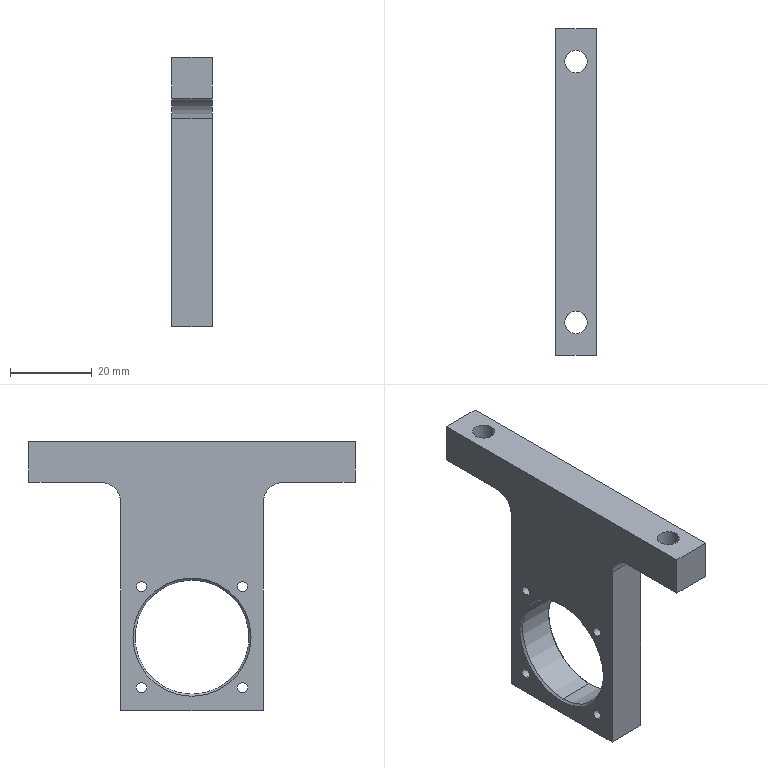Part | SolidWorks | features HoleWzd 2, Chamfer 1, Extrusion 1, Fillet 1, ICE 1 | 1 solid | 30 faces | box 10 x 80 x 66 mm | volume 20856 mm3 | cylinder 16 | plane 10 | cone 4 | commonest cylinder face diameters 2.5 x8 5.5 x4 10 x2 28 x2
STEP:
#1=CARTESIAN_POINT('',(9.5,0.,-34.));
#2=VERTEX_POINT('',#1);
#3=CARTESIAN_POINT('',(9.5,0.,-62.));
#4=VERTEX_POINT('',#3);
#5=CARTESIAN_POINT('',(9.5,0.,-48.));
#6=DIRECTION('',(1.,0.,0.));
#7=DIRECTION('',(0.,0.,1.));
#8=AXIS2_PLACEMENT_3D('',#5,#6,#7);
#9=CIRCLE('',#8,14.);
#10=EDGE_CURVE('',#2,#4,#9,.T.);
#11=ORIENTED_EDGE('',*,*,#10,.F.);
#12=CARTESIAN_POINT('',(10.,0.,-33.5));
#13=VERTEX_POINT('',#12);
#14=CARTESIAN_POINT('',(9.5,0.,-34.));
#15=DIRECTION('',(0.7071,0.,0.7071));
#16=VECTOR('',#15,1000.);
#17=LINE('',#14,#16);
#18=EDGE_CURVE('',#2,#13,#17,.T.);
#19=ORIENTED_EDGE('',*,*,#18,.T.);
#20=CARTESIAN_POINT('',(10.,0.,-62.5));
#21=VERTEX_POINT('',#20);
#22=CARTESIAN_POINT('',(10.,0.,-48.));
#23=DIRECTION('',(-1.,0.,0.));
#24=DIRECTION('',(0.,0.,1.));
#25=AXIS2_PLACEMENT_3D('',#22,#23,#24);
#26=CIRCLE('',#25,14.5);
#27=EDGE_CURVE('',#21,#13,#26,.T.);
#28=ORIENTED_EDGE('',*,*,#27,.F.);
#29=CARTESIAN_POINT('',(9.5,0.,-62.));
#30=DIRECTION('',(0.7071,0.,-0.7071));
#31=VECTOR('',#30,1000.);
#32=LINE('',#29,#31);
#33=EDGE_CURVE('',#4,#21,#32,.T.);
#34=ORIENTED_EDGE('',*,*,#33,.F.);
#35=EDGE_LOOP('',(#11,#19,#28,#34));
#36=FACE_OUTER_BOUND('',#35,.T.);
#37=CARTESIAN_POINT('',(9.5,0.,-48.));
#38=DIRECTION('',(1.,0.,0.));
#39=DIRECTION('',(0.,0.,-1.));
#40=AXIS2_PLACEMENT_3D('',#37,#38,#39);
#41=CONICAL_SURFACE('',#40,14.,0.7854);
#42=ADVANCED_FACE('',(#36),#41,.F.);
#43=CARTESIAN_POINT('',(0.5,0.,-62.));
#44=VERTEX_POINT('',#43);
#45=CARTESIAN_POINT('',(0.5,0.,-34.));
#46=VERTEX_POINT('',#45);
#47=CARTESIAN_POINT('',(0.5,0.,-48.));
#48=DIRECTION('',(-1.,0.,0.));
#49=DIRECTION('',(0.,0.,1.));
#50=AXIS2_PLACEMENT_3D('',#47,#48,#49);
#51=CIRCLE('',#50,14.);
#52=EDGE_CURVE('',#44,#46,#51,.T.);
#53=ORIENTED_EDGE('',*,*,#52,.F.);
#54=CARTESIAN_POINT('',(0.,0.,-62.5));
#55=VERTEX_POINT('',#54);
#56=CARTESIAN_POINT('',(0.,0.,-62.5));
#57=DIRECTION('',(-0.7071,0.,-0.7071));
#58=VECTOR('',#57,1000.);
#59=LINE('',#56,#58);
#60=EDGE_CURVE('',#44,#55,#59,.T.);
#61=ORIENTED_EDGE('',*,*,#60,.T.);
#62=CARTESIAN_POINT('',(0.,0.,-33.5));
#63=VERTEX_POINT('',#62);
#64=CARTESIAN_POINT('',(0.,0.,-48.));
#65=DIRECTION('',(1.,0.,0.));
#66=DIRECTION('',(0.,0.,1.));
#67=AXIS2_PLACEMENT_3D('',#64,#65,#66);
#68=CIRCLE('',#67,14.5);
#69=EDGE_CURVE('',#63,#55,#68,.T.);
#70=ORIENTED_EDGE('',*,*,#69,.F.);
#71=CARTESIAN_POINT('',(0.,0.,-33.5));
#72=DIRECTION('',(-0.7071,0.,0.7071));
#73=VECTOR('',#72,1000.);
#74=LINE('',#71,#73);
#75=EDGE_CURVE('',#46,#63,#74,.T.);
#76=ORIENTED_EDGE('',*,*,#75,.F.);
#77=EDGE_LOOP('',(#53,#61,#70,#76));
#78=FACE_OUTER_BOUND('',#77,.T.);
#79=CARTESIAN_POINT('',(0.,0.,-48.));
#80=DIRECTION('',(-1.,0.,0.));
#81=DIRECTION('',(0.,0.,1.));
#82=AXIS2_PLACEMENT_3D('',#79,#80,#81);
#83=CONICAL_SURFACE('',#82,14.5,0.7854);
#84=ADVANCED_FACE('',(#78),#83,.F.);
#85=CARTESIAN_POINT('',(0.,12.374,-34.376));
#86=VERTEX_POINT('',#85);
#87=CARTESIAN_POINT('',(0.,12.374,-36.876));
#88=VERTEX_POINT('',#87);
#89=CARTESIAN_POINT('',(0.,12.374,-35.626));
#90=DIRECTION('',(1.,0.,0.));
#91=DIRECTION('',(0.,0.,-1.));
#92=AXIS2_PLACEMENT_3D('',#89,#90,#91);
#93=CIRCLE('',#92,1.25);
#94=EDGE_CURVE('',#86,#88,#93,.T.);
#95=ORIENTED_EDGE('',*,*,#94,.F.);
#96=CARTESIAN_POINT('',(10.,12.374,-34.376));
#97=VERTEX_POINT('',#96);
#98=CARTESIAN_POINT('',(10.,12.374,-34.376));
#99=DIRECTION('',(1.,0.,0.));
#100=VECTOR('',#99,1000.);
#101=LINE('',#98,#100);
#102=EDGE_CURVE('',#86,#97,#101,.T.);
#103=ORIENTED_EDGE('',*,*,#102,.T.);
#104=CARTESIAN_POINT('',(10.,12.374,-36.876));
#105=VERTEX_POINT('',#104);
#106=CARTESIAN_POINT('',(10.,12.374,-35.626));
#107=DIRECTION('',(1.,0.,0.));
#108=DIRECTION('',(0.,0.,-1.));
#109=AXIS2_PLACEMENT_3D('',#106,#107,#108);
#110=CIRCLE('',#109,1.25);
#111=EDGE_CURVE('',#97,#105,#110,.T.);
#112=ORIENTED_EDGE('',*,*,#111,.T.);
#113=CARTESIAN_POINT('',(10.,12.374,-36.876));
#114=DIRECTION('',(1.,0.,0.));
#115=VECTOR('',#114,1000.);
#116=LINE('',#113,#115);
#117=EDGE_CURVE('',#88,#105,#116,.T.);
#118=ORIENTED_EDGE('',*,*,#117,.F.);
#119=EDGE_LOOP('',(#95,#103,#112,#118));
#120=FACE_OUTER_BOUND('',#119,.T.);
#121=CARTESIAN_POINT('',(10.,12.374,-35.626));
#122=DIRECTION('',(1.,0.,0.));
#123=DIRECTION('',(0.,0.,-1.));
#124=AXIS2_PLACEMENT_3D('',#121,#122,#123);
#125=CYLINDRICAL_SURFACE('',#124,1.25);
#126=ADVANCED_FACE('',(#120),#125,.F.);
#127=CARTESIAN_POINT('',(0.,12.374,-59.124));
#128=VERTEX_POINT('',#127);
#129=CARTESIAN_POINT('',(0.,12.374,-61.624));
#130=VERTEX_POINT('',#129);
#131=CARTESIAN_POINT('',(0.,12.374,-60.374));
#132=DIRECTION('',(1.,0.,0.));
#133=DIRECTION('',(0.,0.,-1.));
#134=AXIS2_PLACEMENT_3D('',#131,#132,#133);
#135=CIRCLE('',#134,1.25);
#136=EDGE_CURVE('',#128,#130,#135,.T.);
#137=ORIENTED_EDGE('',*,*,#136,.F.);
#138=CARTESIAN_POINT('',(10.,12.374,-59.124));
#139=VERTEX_POINT('',#138);
#140=CARTESIAN_POINT('',(10.,12.374,-59.124));
#141=DIRECTION('',(1.,0.,0.));
#142=VECTOR('',#141,1000.);
#143=LINE('',#140,#142);
#144=EDGE_CURVE('',#128,#139,#143,.T.);
#145=ORIENTED_EDGE('',*,*,#144,.T.);
#146=CARTESIAN_POINT('',(10.,12.374,-61.624));
#147=VERTEX_POINT('',#146);
#148=CARTESIAN_POINT('',(10.,12.374,-60.374));
#149=DIRECTION('',(1.,0.,0.));
#150=DIRECTION('',(0.,0.,-1.));
#151=AXIS2_PLACEMENT_3D('',#148,#149,#150);
#152=CIRCLE('',#151,1.25);
#153=EDGE_CURVE('',#139,#147,#152,.T.);
#154=ORIENTED_EDGE('',*,*,#153,.T.);
#155=CARTESIAN_POINT('',(10.,12.374,-61.624));
#156=DIRECTION('',(1.,0.,0.));
#157=VECTOR('',#156,1000.);
#158=LINE('',#155,#157);
#159=EDGE_CURVE('',#130,#147,#158,.T.);
#160=ORIENTED_EDGE('',*,*,#159,.F.);
#161=EDGE_LOOP('',(#137,#145,#154,#160));
#162=FACE_OUTER_BOUND('',#161,.T.);
#163=CARTESIAN_POINT('',(10.,12.374,-60.374));
#164=DIRECTION('',(1.,0.,0.));
#165=DIRECTION('',(0.,0.,-1.));
#166=AXIS2_PLACEMENT_3D('',#163,#164,#165);
#167=CYLINDRICAL_SURFACE('',#166,1.25);
#168=ADVANCED_FACE('',(#162),#167,.F.);
#169=CARTESIAN_POINT('',(0.,-12.374,-59.124));
#170=VERTEX_POINT('',#169);
#171=CARTESIAN_POINT('',(0.,-12.374,-61.624));
#172=VERTEX_POINT('',#171);
#173=CARTESIAN_POINT('',(0.,-12.374,-60.374));
#174=DIRECTION('',(1.,0.,0.));
#175=DIRECTION('',(0.,0.,-1.));
#176=AXIS2_PLACEMENT_3D('',#173,#174,#175);
#177=CIRCLE('',#176,1.25);
#178=EDGE_CURVE('',#170,#172,#177,.T.);
#179=ORIENTED_EDGE('',*,*,#178,.F.);
#180=CARTESIAN_POINT('',(10.,-12.374,-59.124));
#181=VERTEX_POINT('',#180);
#182=CARTESIAN_POINT('',(10.,-12.374,-59.124));
#183=DIRECTION('',(1.,0.,0.));
#184=VECTOR('',#183,1000.);
#185=LINE('',#182,#184);
#186=EDGE_CURVE('',#170,#181,#185,.T.);
#187=ORIENTED_EDGE('',*,*,#186,.T.);
#188=CARTESIAN_POINT('',(10.,-12.374,-61.624));
#189=VERTEX_POINT('',#188);
#190=CARTESIAN_POINT('',(10.,-12.374,-60.374));
#191=DIRECTION('',(1.,0.,0.));
#192=DIRECTION('',(0.,0.,-1.));
#193=AXIS2_PLACEMENT_3D('',#190,#191,#192);
#194=CIRCLE('',#193,1.25);
#195=EDGE_CURVE('',#181,#189,#194,.T.);
#196=ORIENTED_EDGE('',*,*,#195,.T.);
#197=CARTESIAN_POINT('',(10.,-12.374,-61.624));
#198=DIRECTION('',(1.,0.,0.));
#199=VECTOR('',#198,1000.);
#200=LINE('',#197,#199);
#201=EDGE_CURVE('',#172,#189,#200,.T.);
#202=ORIENTED_EDGE('',*,*,#201,.F.);
#203=EDGE_LOOP('',(#179,#187,#196,#202));
#204=FACE_OUTER_BOUND('',#203,.T.);
#205=CARTESIAN_POINT('',(10.,-12.374,-60.374));
#206=DIRECTION('',(1.,0.,0.));
#207=DIRECTION('',(0.,0.,-1.));
#208=AXIS2_PLACEMENT_3D('',#205,#206,#207);
#209=CYLINDRICAL_SURFACE('',#208,1.25);
#210=ADVANCED_FACE('',(#204),#209,.F.);
#211=CARTESIAN_POINT('',(0.,-12.374,-34.376));
#212=VERTEX_POINT('',#211);
#213=CARTESIAN_POINT('',(0.,-12.374,-36.876));
#214=VERTEX_POINT('',#213);
#215=CARTESIAN_POINT('',(0.,-12.374,-35.626));
#216=DIRECTION('',(1.,0.,0.));
#217=DIRECTION('',(0.,0.,-1.));
#218=AXIS2_PLACEMENT_3D('',#215,#216,#217);
#219=CIRCLE('',#218,1.25);
#220=EDGE_CURVE('',#212,#214,#219,.T.);
#221=ORIENTED_EDGE('',*,*,#220,.F.);
#222=CARTESIAN_POINT('',(10.,-12.374,-34.376));
#223=VERTEX_POINT('',#222);
#224=CARTESIAN_POINT('',(10.,-12.374,-34.376));
#225=DIRECTION('',(1.,0.,0.));
#226=VECTOR('',#225,1000.);
#227=LINE('',#224,#226);
#228=EDGE_CURVE('',#212,#223,#227,.T.);
#229=ORIENTED_EDGE('',*,*,#228,.T.);
#230=CARTESIAN_POINT('',(10.,-12.374,-36.876));
#231=VERTEX_POINT('',#230);
#232=CARTESIAN_POINT('',(10.,-12.374,-35.626));
#233=DIRECTION('',(1.,0.,0.));
#234=DIRECTION('',(0.,0.,-1.));
#235=AXIS2_PLACEMENT_3D('',#232,#233,#234);
#236=CIRCLE('',#235,1.25);
#237=EDGE_CURVE('',#223,#231,#236,.T.);
#238=ORIENTED_EDGE('',*,*,#237,.T.);
#239=CARTESIAN_POINT('',(10.,-12.374,-36.876));
#240=DIRECTION('',(1.,0.,0.));
#241=VECTOR('',#240,1000.);
#242=LINE('',#239,#241);
#243=EDGE_CURVE('',#214,#231,#242,.T.);
#244=ORIENTED_EDGE('',*,*,#243,.F.);
#245=EDGE_LOOP('',(#221,#229,#238,#244));
#246=FACE_OUTER_BOUND('',#245,.T.);
#247=CARTESIAN_POINT('',(10.,-12.374,-35.626));
#248=DIRECTION('',(1.,0.,0.));
#249=DIRECTION('',(0.,0.,-1.));
#250=AXIS2_PLACEMENT_3D('',#247,#248,#249);
#251=CYLINDRICAL_SURFACE('',#250,1.25);
#252=ADVANCED_FACE('',(#246),#251,.F.);
#253=CARTESIAN_POINT('',(2.25,32.,-10.));
#254=VERTEX_POINT('',#253);
#255=CARTESIAN_POINT('',(7.75,32.,-10.));
#256=VERTEX_POINT('',#255);
#257=CARTESIAN_POINT('',(5.,32.,-10.));
#258=DIRECTION('',(0.,0.,1.));
#259=DIRECTION('',(1.,0.,0.));
#260=AXIS2_PLACEMENT_3D('',#257,#258,#259);
#261=CIRCLE('',#260,2.75);
#262=EDGE_CURVE('',#254,#256,#261,.T.);
#263=ORIENTED_EDGE('',*,*,#262,.F.);
#264=CARTESIAN_POINT('',(2.25,32.,0.));
#265=VERTEX_POINT('',#264);
#266=CARTESIAN_POINT('',(2.25,32.,0.));
#267=DIRECTION('',(0.,0.,1.));
#268=VECTOR('',#267,1000.);
#269=LINE('',#266,#268);
#270=EDGE_CURVE('',#254,#265,#269,.T.);
#271=ORIENTED_EDGE('',*,*,#270,.T.);
#272=CARTESIAN_POINT('',(7.75,32.,0.));
#273=VERTEX_POINT('',#272);
#274=CARTESIAN_POINT('',(5.,32.,0.));
#275=DIRECTION('',(0.,0.,1.));
#276=DIRECTION('',(1.,0.,0.));
#277=AXIS2_PLACEMENT_3D('',#274,#275,#276);
#278=CIRCLE('',#277,2.75);
#279=EDGE_CURVE('',#265,#273,#278,.T.);
#280=ORIENTED_EDGE('',*,*,#279,.T.);
#281=CARTESIAN_POINT('',(7.75,32.,0.));
#282=DIRECTION('',(0.,0.,1.));
#283=VECTOR('',#282,1000.);
#284=LINE('',#281,#283);
#285=EDGE_CURVE('',#256,#273,#284,.T.);
#286=ORIENTED_EDGE('',*,*,#285,.F.);
#287=EDGE_LOOP('',(#263,#271,#280,#286));
#288=FACE_OUTER_BOUND('',#287,.T.);
#289=CARTESIAN_POINT('',(5.,32.,0.));
#290=DIRECTION('',(0.,0.,1.));
#291=DIRECTION('',(1.,0.,0.));
#292=AXIS2_PLACEMENT_3D('',#289,#290,#291);
#293=CYLINDRICAL_SURFACE('',#292,2.75);
#294=ADVANCED_FACE('',(#288),#293,.F.);
#295=CARTESIAN_POINT('',(2.25,-32.,-10.));
#296=VERTEX_POINT('',#295);
#297=CARTESIAN_POINT('',(7.75,-32.,-10.));
#298=VERTEX_POINT('',#297);
#299=CARTESIAN_POINT('',(5.,-32.,-10.));
#300=DIRECTION('',(0.,0.,1.));
#301=DIRECTION('',(1.,0.,0.));
#302=AXIS2_PLACEMENT_3D('',#299,#300,#301);
#303=CIRCLE('',#302,2.75);
#304=EDGE_CURVE('',#296,#298,#303,.T.);
#305=ORIENTED_EDGE('',*,*,#304,.F.);
#306=CARTESIAN_POINT('',(2.25,-32.,0.));
#307=VERTEX_POINT('',#306);
#308=CARTESIAN_POINT('',(2.25,-32.,0.));
#309=DIRECTION('',(0.,0.,1.));
#310=VECTOR('',#309,1000.);
#311=LINE('',#308,#310);
#312=EDGE_CURVE('',#296,#307,#311,.T.);
#313=ORIENTED_EDGE('',*,*,#312,.T.);
#314=CARTESIAN_POINT('',(7.75,-32.,0.));
#315=VERTEX_POINT('',#314);
#316=CARTESIAN_POINT('',(5.,-32.,0.));
#317=DIRECTION('',(0.,0.,1.));
#318=DIRECTION('',(1.,0.,0.));
#319=AXIS2_PLACEMENT_3D('',#316,#317,#318);
#320=CIRCLE('',#319,2.75);
#321=EDGE_CURVE('',#307,#315,#320,.T.);
#322=ORIENTED_EDGE('',*,*,#321,.T.);
#323=CARTESIAN_POINT('',(7.75,-32.,0.));
#324=DIRECTION('',(0.,0.,1.));
#325=VECTOR('',#324,1000.);
#326=LINE('',#323,#325);
#327=EDGE_CURVE('',#298,#315,#326,.T.);
#328=ORIENTED_EDGE('',*,*,#327,.F.);
#329=EDGE_LOOP('',(#305,#313,#322,#328));
#330=FACE_OUTER_BOUND('',#329,.T.);
#331=CARTESIAN_POINT('',(5.,-32.,0.));
#332=DIRECTION('',(0.,0.,1.));
#333=DIRECTION('',(1.,0.,0.));
#334=AXIS2_PLACEMENT_3D('',#331,#332,#333);
#335=CYLINDRICAL_SURFACE('',#334,2.75);
#336=ADVANCED_FACE('',(#330),#335,.F.);
#337=ORIENTED_EDGE('',*,*,#52,.T.);
#338=CARTESIAN_POINT('',(0.,0.,-34.));
#339=DIRECTION('',(1.,0.,0.));
#340=VECTOR('',#339,1000.);
#341=LINE('',#338,#340);
#342=EDGE_CURVE('',#46,#2,#341,.T.);
#343=ORIENTED_EDGE('',*,*,#342,.T.);
#344=ORIENTED_EDGE('',*,*,#10,.T.);
#345=CARTESIAN_POINT('',(0.,0.,-62.));
#346=DIRECTION('',(1.,0.,0.));
#347=VECTOR('',#346,1000.);
#348=LINE('',#345,#347);
#349=EDGE_CURVE('',#44,#4,#348,.T.);
#350=ORIENTED_EDGE('',*,*,#349,.F.);
#351=EDGE_LOOP('',(#337,#343,#344,#350));
#352=FACE_OUTER_BOUND('',#351,.T.);
#353=CARTESIAN_POINT('',(0.,0.,-48.));
#354=DIRECTION('',(1.,0.,0.));
#355=DIRECTION('',(0.,0.,-1.));
#356=AXIS2_PLACEMENT_3D('',#353,#354,#355);
#357=CYLINDRICAL_SURFACE('',#356,14.);
#358=ADVANCED_FACE('',(#352),#357,.F.);
#359=CARTESIAN_POINT('',(0.,-40.,0.));
#360=VERTEX_POINT('',#359);
#361=CARTESIAN_POINT('',(0.,-40.,-10.));
#362=VERTEX_POINT('',#361);
#363=CARTESIAN_POINT('',(0.,-40.,-10.));
#364=DIRECTION('',(0.,0.,-1.));
#365=VECTOR('',#364,1000.);
#366=LINE('',#363,#365);
#367=EDGE_CURVE('',#360,#362,#366,.T.);
#368=ORIENTED_EDGE('',*,*,#367,.T.);
#369=CARTESIAN_POINT('',(10.,-40.,-10.));
#370=VERTEX_POINT('',#369);
#371=CARTESIAN_POINT('',(10.,-40.,-10.));
#372=DIRECTION('',(-1.,0.,0.));
#373=VECTOR('',#372,1000.);
#374=LINE('',#371,#373);
#375=EDGE_CURVE('',#370,#362,#374,.T.);
#376=ORIENTED_EDGE('',*,*,#375,.F.);
#377=CARTESIAN_POINT('',(10.,-40.,0.));
#378=VERTEX_POINT('',#377);
#379=CARTESIAN_POINT('',(10.,-40.,-10.));
#380=DIRECTION('',(0.,0.,-1.));
#381=VECTOR('',#380,1000.);
#382=LINE('',#379,#381);
#383=EDGE_CURVE('',#378,#370,#382,.T.);
#384=ORIENTED_EDGE('',*,*,#383,.F.);
#385=CARTESIAN_POINT('',(10.,-40.,0.));
#386=DIRECTION('',(-1.,0.,0.));
#387=VECTOR('',#386,1000.);
#388=LINE('',#385,#387);
#389=EDGE_CURVE('',#378,#360,#388,.T.);
#390=ORIENTED_EDGE('',*,*,#389,.T.);
#391=EDGE_LOOP('',(#368,#376,#384,#390));
#392=FACE_OUTER_BOUND('',#391,.T.);
#393=CARTESIAN_POINT('',(10.,-40.,-10.));
#394=DIRECTION('',(0.,1.,0.));
#395=DIRECTION('',(0.,0.,1.));
#396=AXIS2_PLACEMENT_3D('',#393,#394,#395);
#397=PLANE('',#396);
#398=ADVANCED_FACE('',(#392),#397,.F.);
#399=CARTESIAN_POINT('',(5.,-32.,-10.));
#400=DIRECTION('',(0.,0.,1.));
#401=DIRECTION('',(1.,0.,0.));
#402=AXIS2_PLACEMENT_3D('',#399,#400,#401);
#403=CIRCLE('',#402,2.75);
#404=EDGE_CURVE('',#298,#296,#403,.T.);
#405=ORIENTED_EDGE('',*,*,#404,.T.);
#406=ORIENTED_EDGE('',*,*,#304,.T.);
#407=EDGE_LOOP('',(#405,#406));
#408=FACE_BOUND('',#407,.T.);
#409=CARTESIAN_POINT('',(0.,-22.5,-10.));
#410=VERTEX_POINT('',#409);
#411=CARTESIAN_POINT('',(0.,-17.5,-10.));
#412=DIRECTION('',(0.,1.,0.));
#413=VECTOR('',#412,1000.);
#414=LINE('',#411,#413);
#415=EDGE_CURVE('',#362,#410,#414,.T.);
#416=ORIENTED_EDGE('',*,*,#415,.T.);
#417=CARTESIAN_POINT('',(10.,-22.5,-10.));
#418=VERTEX_POINT('',#417);
#419=CARTESIAN_POINT('',(10.,-22.5,-10.));
#420=DIRECTION('',(1.,0.,0.));
#421=VECTOR('',#420,1000.);
#422=LINE('',#419,#421);
#423=EDGE_CURVE('',#410,#418,#422,.T.);
#424=ORIENTED_EDGE('',*,*,#423,.T.);
#425=CARTESIAN_POINT('',(10.,-17.5,-10.));
#426=DIRECTION('',(0.,1.,0.));
#427=VECTOR('',#426,1000.);
#428=LINE('',#425,#427);
#429=EDGE_CURVE('',#370,#418,#428,.T.);
#430=ORIENTED_EDGE('',*,*,#429,.F.);
#431=ORIENTED_EDGE('',*,*,#375,.T.);
#432=EDGE_LOOP('',(#416,#424,#430,#431));
#433=FACE_OUTER_BOUND('',#432,.T.);
#434=CARTESIAN_POINT('',(10.,-17.5,-10.));
#435=DIRECTION('',(0.,0.,1.));
#436=DIRECTION('',(1.,0.,0.));
#437=AXIS2_PLACEMENT_3D('',#434,#435,#436);
#438=PLANE('',#437);
#439=ADVANCED_FACE('',(#408,#433),#438,.F.);
#440=CARTESIAN_POINT('',(10.,-17.5,-15.));
#441=VERTEX_POINT('',#440);
#442=CARTESIAN_POINT('',(10.,-17.5,-66.));
#443=VERTEX_POINT('',#442);
#444=CARTESIAN_POINT('',(10.,-17.5,-66.));
#445=DIRECTION('',(0.,0.,-1.));
#446=VECTOR('',#445,1000.);
#447=LINE('',#444,#446);
#448=EDGE_CURVE('',#441,#443,#447,.T.);
#449=ORIENTED_EDGE('',*,*,#448,.F.);
#450=CARTESIAN_POINT('',(0.,-17.5,-15.));
#451=VERTEX_POINT('',#450);
#452=CARTESIAN_POINT('',(0.,-17.5,-15.));
#453=DIRECTION('',(-1.,0.,0.));
#454=VECTOR('',#453,1000.);
#455=LINE('',#452,#454);
#456=EDGE_CURVE('',#441,#451,#455,.T.);
#457=ORIENTED_EDGE('',*,*,#456,.T.);
#458=CARTESIAN_POINT('',(0.,-17.5,-66.));
#459=VERTEX_POINT('',#458);
#460=CARTESIAN_POINT('',(0.,-17.5,-66.));
#461=DIRECTION('',(0.,0.,-1.));
#462=VECTOR('',#461,1000.);
#463=LINE('',#460,#462);
#464=EDGE_CURVE('',#451,#459,#463,.T.);
#465=ORIENTED_EDGE('',*,*,#464,.T.);
#466=CARTESIAN_POINT('',(10.,-17.5,-66.));
#467=DIRECTION('',(-1.,0.,0.));
#468=VECTOR('',#467,1000.);
#469=LINE('',#466,#468);
#470=EDGE_CURVE('',#443,#459,#469,.T.);
#471=ORIENTED_EDGE('',*,*,#470,.F.);
#472=EDGE_LOOP('',(#449,#457,#465,#471));
#473=FACE_OUTER_BOUND('',#472,.T.);
#474=CARTESIAN_POINT('',(10.,-17.5,-66.));
#475=DIRECTION('',(0.,1.,0.));
#476=DIRECTION('',(0.,0.,1.));
#477=AXIS2_PLACEMENT_3D('',#474,#475,#476);
#478=PLANE('',#477);
#479=ADVANCED_FACE('',(#473),#478,.F.);
#480=CARTESIAN_POINT('',(0.,17.5,-66.));
#481=VERTEX_POINT('',#480);
#482=CARTESIAN_POINT('',(0.,17.5,-66.));
#483=DIRECTION('',(0.,1.,0.));
#484=VECTOR('',#483,1000.);
#485=LINE('',#482,#484);
#486=EDGE_CURVE('',#459,#481,#485,.T.);
#487=ORIENTED_EDGE('',*,*,#486,.T.);
#488=CARTESIAN_POINT('',(10.,17.5,-66.));
#489=VERTEX_POINT('',#488);
#490=CARTESIAN_POINT('',(10.,17.5,-66.));
#491=DIRECTION('',(-1.,0.,0.));
#492=VECTOR('',#491,1000.);
#493=LINE('',#490,#492);
#494=EDGE_CURVE('',#489,#481,#493,.T.);
#495=ORIENTED_EDGE('',*,*,#494,.F.);
#496=CARTESIAN_POINT('',(10.,17.5,-66.));
#497=DIRECTION('',(0.,1.,0.));
#498=VECTOR('',#497,1000.);
#499=LINE('',#496,#498);
#500=EDGE_CURVE('',#443,#489,#499,.T.);
#501=ORIENTED_EDGE('',*,*,#500,.F.);
#502=ORIENTED_EDGE('',*,*,#470,.T.);
#503=EDGE_LOOP('',(#487,#495,#501,#502));
#504=FACE_OUTER_BOUND('',#503,.T.);
#505=CARTESIAN_POINT('',(10.,17.5,-66.));
#506=DIRECTION('',(0.,0.,1.));
#507=DIRECTION('',(1.,0.,0.));
#508=AXIS2_PLACEMENT_3D('',#505,#506,#507);
#509=PLANE('',#508);
#510=ADVANCED_FACE('',(#504),#509,.F.);
#511=CARTESIAN_POINT('',(0.,17.5,-15.));
#512=VERTEX_POINT('',#511);
#513=CARTESIAN_POINT('',(0.,17.5,-10.));
#514=DIRECTION('',(0.,0.,1.));
#515=VECTOR('',#514,1000.);
#516=LINE('',#513,#515);
#517=EDGE_CURVE('',#481,#512,#516,.T.);
#518=ORIENTED_EDGE('',*,*,#517,.T.);
#519=CARTESIAN_POINT('',(10.,17.5,-15.));
#520=VERTEX_POINT('',#519);
#521=CARTESIAN_POINT('',(10.,17.5,-15.));
#522=DIRECTION('',(1.,0.,0.));
#523=VECTOR('',#522,1000.);
#524=LINE('',#521,#523);
#525=EDGE_CURVE('',#512,#520,#524,.T.);
#526=ORIENTED_EDGE('',*,*,#525,.T.);
#527=CARTESIAN_POINT('',(10.,17.5,-10.));
#528=DIRECTION('',(0.,0.,1.));
#529=VECTOR('',#528,1000.);
#530=LINE('',#527,#529);
#531=EDGE_CURVE('',#489,#520,#530,.T.);
#532=ORIENTED_EDGE('',*,*,#531,.F.);
#533=ORIENTED_EDGE('',*,*,#494,.T.);
#534=EDGE_LOOP('',(#518,#526,#532,#533));
#535=FACE_OUTER_BOUND('',#534,.T.);
#536=CARTESIAN_POINT('',(10.,17.5,-10.));
#537=DIRECTION('',(0.,-1.,0.));
#538=DIRECTION('',(0.,0.,-1.));
#539=AXIS2_PLACEMENT_3D('',#536,#537,#538);
#540=PLANE('',#539);
#541=ADVANCED_FACE('',(#535),#540,.F.);
#542=CARTESIAN_POINT('',(5.,32.,-10.));
#543=DIRECTION('',(0.,0.,1.));
#544=DIRECTION('',(1.,0.,0.));
#545=AXIS2_PLACEMENT_3D('',#542,#543,#544);
#546=CIRCLE('',#545,2.75);
#547=EDGE_CURVE('',#256,#254,#546,.T.);
#548=ORIENTED_EDGE('',*,*,#547,.T.);
#549=ORIENTED_EDGE('',*,*,#262,.T.);
#550=EDGE_LOOP('',(#548,#549));
#551=FACE_BOUND('',#550,.T.);
#552=CARTESIAN_POINT('',(10.,22.5,-10.));
#553=VERTEX_POINT('',#552);
#554=CARTESIAN_POINT('',(10.,40.,-10.));
#555=VERTEX_POINT('',#554);
#556=CARTESIAN_POINT('',(10.,40.,-10.));
#557=DIRECTION('',(0.,1.,0.));
#558=VECTOR('',#557,1000.);
#559=LINE('',#556,#558);
#560=EDGE_CURVE('',#553,#555,#559,.T.);
#561=ORIENTED_EDGE('',*,*,#560,.F.);
#562=CARTESIAN_POINT('',(0.,22.5,-10.));
#563=VERTEX_POINT('',#562);
#564=CARTESIAN_POINT('',(0.,22.5,-10.));
#565=DIRECTION('',(-1.,0.,0.));
#566=VECTOR('',#565,1000.);
#567=LINE('',#564,#566);
#568=EDGE_CURVE('',#553,#563,#567,.T.);
#569=ORIENTED_EDGE('',*,*,#568,.T.);
#570=CARTESIAN_POINT('',(0.,40.,-10.));
#571=VERTEX_POINT('',#570);
#572=CARTESIAN_POINT('',(0.,40.,-10.));
#573=DIRECTION('',(0.,1.,0.));
#574=VECTOR('',#573,1000.);
#575=LINE('',#572,#574);
#576=EDGE_CURVE('',#563,#571,#575,.T.);
#577=ORIENTED_EDGE('',*,*,#576,.T.);
#578=CARTESIAN_POINT('',(10.,40.,-10.));
#579=DIRECTION('',(-1.,0.,0.));
#580=VECTOR('',#579,1000.);
#581=LINE('',#578,#580);
#582=EDGE_CURVE('',#555,#571,#581,.T.);
#583=ORIENTED_EDGE('',*,*,#582,.F.);
#584=EDGE_LOOP('',(#561,#569,#577,#583));
#585=FACE_OUTER_BOUND('',#584,.T.);
#586=CARTESIAN_POINT('',(10.,40.,-10.));
#587=DIRECTION('',(0.,0.,1.));
#588=DIRECTION('',(1.,0.,0.));
#589=AXIS2_PLACEMENT_3D('',#586,#587,#588);
#590=PLANE('',#589);
#591=ADVANCED_FACE('',(#551,#585),#590,.F.);
#592=CARTESIAN_POINT('',(0.,40.,0.));
#593=VERTEX_POINT('',#592);
#594=CARTESIAN_POINT('',(0.,40.,0.));
#595=DIRECTION('',(0.,0.,1.));
#596=VECTOR('',#595,1000.);
#597=LINE('',#594,#596);
#598=EDGE_CURVE('',#571,#593,#597,.T.);
#599=ORIENTED_EDGE('',*,*,#598,.T.);
#600=CARTESIAN_POINT('',(10.,40.,0.));
#601=VERTEX_POINT('',#600);
#602=CARTESIAN_POINT('',(10.,40.,0.));
#603=DIRECTION('',(-1.,0.,0.));
#604=VECTOR('',#603,1000.);
#605=LINE('',#602,#604);
#606=EDGE_CURVE('',#601,#593,#605,.T.);
#607=ORIENTED_EDGE('',*,*,#606,.F.);
#608=CARTESIAN_POINT('',(10.,40.,0.));
#609=DIRECTION('',(0.,0.,1.));
#610=VECTOR('',#609,1000.);
#611=LINE('',#608,#610);
#612=EDGE_CURVE('',#555,#601,#611,.T.);
#613=ORIENTED_EDGE('',*,*,#612,.F.);
#614=ORIENTED_EDGE('',*,*,#582,.T.);
#615=EDGE_LOOP('',(#599,#607,#613,#614));
#616=FACE_OUTER_BOUND('',#615,.T.);
#617=CARTESIAN_POINT('',(10.,40.,0.));
#618=DIRECTION('',(0.,-1.,0.));
#619=DIRECTION('',(0.,0.,-1.));
#620=AXIS2_PLACEMENT_3D('',#617,#618,#619);
#621=PLANE('',#620);
#622=ADVANCED_FACE('',(#616),#621,.F.);
#623=CARTESIAN_POINT('',(5.,32.,0.));
#624=DIRECTION('',(0.,0.,1.));
#625=DIRECTION('',(1.,0.,0.));
#626=AXIS2_PLACEMENT_3D('',#623,#624,#625);
#627=CIRCLE('',#626,2.75);
#628=EDGE_CURVE('',#273,#265,#627,.T.);
#629=ORIENTED_EDGE('',*,*,#628,.F.);
#630=ORIENTED_EDGE('',*,*,#279,.F.);
#631=EDGE_LOOP('',(#629,#630));
#632=FACE_BOUND('',#631,.T.);
#633=CARTESIAN_POINT('',(5.,-32.,0.));
#634=DIRECTION('',(0.,0.,1.));
#635=DIRECTION('',(1.,0.,0.));
#636=AXIS2_PLACEMENT_3D('',#633,#634,#635);
#637=CIRCLE('',#636,2.75);
#638=EDGE_CURVE('',#315,#307,#637,.T.);
#639=ORIENTED_EDGE('',*,*,#638,.F.);
#640=ORIENTED_EDGE('',*,*,#321,.F.);
#641=EDGE_LOOP('',(#639,#640));
#642=FACE_BOUND('',#641,.T.);
#643=CARTESIAN_POINT('',(0.,-40.,0.));
#644=DIRECTION('',(0.,-1.,0.));
#645=VECTOR('',#644,1000.);
#646=LINE('',#643,#645);
#647=EDGE_CURVE('',#593,#360,#646,.T.);
#648=ORIENTED_EDGE('',*,*,#647,.T.);
#649=ORIENTED_EDGE('',*,*,#389,.F.);
#650=CARTESIAN_POINT('',(10.,-40.,0.));
#651=DIRECTION('',(0.,-1.,0.));
#652=VECTOR('',#651,1000.);
#653=LINE('',#650,#652);
#654=EDGE_CURVE('',#601,#378,#653,.T.);
#655=ORIENTED_EDGE('',*,*,#654,.F.);
#656=ORIENTED_EDGE('',*,*,#606,.T.);
#657=EDGE_LOOP('',(#648,#649,#655,#656));
#658=FACE_OUTER_BOUND('',#657,.T.);
#659=CARTESIAN_POINT('',(10.,-40.,0.));
#660=DIRECTION('',(0.,0.,-1.));
#661=DIRECTION('',(-1.,0.,0.));
#662=AXIS2_PLACEMENT_3D('',#659,#660,#661);
#663=PLANE('',#662);
#664=ADVANCED_FACE('',(#632,#642,#658),#663,.F.);
#665=ORIENTED_EDGE('',*,*,#27,.T.);
#666=CARTESIAN_POINT('',(10.,0.,-48.));
#667=DIRECTION('',(-1.,0.,0.));
#668=DIRECTION('',(0.,0.,1.));
#669=AXIS2_PLACEMENT_3D('',#666,#667,#668);
#670=CIRCLE('',#669,14.5);
#671=EDGE_CURVE('',#13,#21,#670,.T.);
#672=ORIENTED_EDGE('',*,*,#671,.T.);
#673=EDGE_LOOP('',(#665,#672));
#674=FACE_BOUND('',#673,.T.);
#675=CARTESIAN_POINT('',(10.,12.374,-35.626));
#676=DIRECTION('',(1.,0.,0.));
#677=DIRECTION('',(0.,0.,-1.));
#678=AXIS2_PLACEMENT_3D('',#675,#676,#677);
#679=CIRCLE('',#678,1.25);
#680=EDGE_CURVE('',#105,#97,#679,.T.);
#681=ORIENTED_EDGE('',*,*,#680,.F.);
#682=ORIENTED_EDGE('',*,*,#111,.F.);
#683=EDGE_LOOP('',(#681,#682));
#684=FACE_BOUND('',#683,.T.);
#685=CARTESIAN_POINT('',(10.,12.374,-60.374));
#686=DIRECTION('',(1.,0.,0.));
#687=DIRECTION('',(0.,0.,-1.));
#688=AXIS2_PLACEMENT_3D('',#685,#686,#687);
#689=CIRCLE('',#688,1.25);
#690=EDGE_CURVE('',#147,#139,#689,.T.);
#691=ORIENTED_EDGE('',*,*,#690,.F.);
#692=ORIENTED_EDGE('',*,*,#153,.F.);
#693=EDGE_LOOP('',(#691,#692));
#694=FACE_BOUND('',#693,.T.);
#695=CARTESIAN_POINT('',(10.,-12.374,-60.374));
#696=DIRECTION('',(1.,0.,0.));
#697=DIRECTION('',(0.,0.,-1.));
#698=AXIS2_PLACEMENT_3D('',#695,#696,#697);
#699=CIRCLE('',#698,1.25);
#700=EDGE_CURVE('',#189,#181,#699,.T.);
#701=ORIENTED_EDGE('',*,*,#700,.F.);
#702=ORIENTED_EDGE('',*,*,#195,.F.);
#703=EDGE_LOOP('',(#701,#702));
#704=FACE_BOUND('',#703,.T.);
#705=CARTESIAN_POINT('',(10.,-12.374,-35.626));
#706=DIRECTION('',(1.,0.,0.));
#707=DIRECTION('',(0.,0.,-1.));
#708=AXIS2_PLACEMENT_3D('',#705,#706,#707);
#709=CIRCLE('',#708,1.25);
#710=EDGE_CURVE('',#231,#223,#709,.T.);
#711=ORIENTED_EDGE('',*,*,#710,.F.);
#712=ORIENTED_EDGE('',*,*,#237,.F.);
#713=EDGE_LOOP('',(#711,#712));
#714=FACE_BOUND('',#713,.T.);
#715=ORIENTED_EDGE('',*,*,#383,.T.);
#716=ORIENTED_EDGE('',*,*,#429,.T.);
#717=CARTESIAN_POINT('',(10.,-22.5,-15.));
#718=DIRECTION('',(-1.,0.,0.));
#719=DIRECTION('',(0.,0.,1.));
#720=AXIS2_PLACEMENT_3D('',#717,#718,#719);
#721=CIRCLE('',#720,5.);
#722=EDGE_CURVE('',#418,#441,#721,.T.);
#723=ORIENTED_EDGE('',*,*,#722,.T.);
#724=ORIENTED_EDGE('',*,*,#448,.T.);
#725=ORIENTED_EDGE('',*,*,#500,.T.);
#726=ORIENTED_EDGE('',*,*,#531,.T.);
#727=CARTESIAN_POINT('',(10.,22.5,-15.));
#728=DIRECTION('',(-1.,0.,0.));
#729=DIRECTION('',(0.,0.,1.));
#730=AXIS2_PLACEMENT_3D('',#727,#728,#729);
#731=CIRCLE('',#730,5.);
#732=EDGE_CURVE('',#520,#553,#731,.T.);
#733=ORIENTED_EDGE('',*,*,#732,.T.);
#734=ORIENTED_EDGE('',*,*,#560,.T.);
#735=ORIENTED_EDGE('',*,*,#612,.T.);
#736=ORIENTED_EDGE('',*,*,#654,.T.);
#737=EDGE_LOOP('',(#715,#716,#723,#724,#725,#726,#733,#734,#735,#736));
#738=FACE_OUTER_BOUND('',#737,.T.);
#739=CARTESIAN_POINT('',(10.,-40.,0.));
#740=DIRECTION('',(-1.,0.,0.));
#741=DIRECTION('',(0.,0.,1.));
#742=AXIS2_PLACEMENT_3D('',#739,#740,#741);
#743=PLANE('',#742);
#744=ADVANCED_FACE('',(#674,#684,#694,#704,#714,#738),#743,.F.);
#745=ORIENTED_EDGE('',*,*,#69,.T.);
#746=CARTESIAN_POINT('',(0.,0.,-48.));
#747=DIRECTION('',(1.,0.,0.));
#748=DIRECTION('',(0.,0.,1.));
#749=AXIS2_PLACEMENT_3D('',#746,#747,#748);
#750=CIRCLE('',#749,14.5);
#751=EDGE_CURVE('',#55,#63,#750,.T.);
#752=ORIENTED_EDGE('',*,*,#751,.T.);
#753=EDGE_LOOP('',(#745,#752));
#754=FACE_BOUND('',#753,.T.);
#755=CARTESIAN_POINT('',(0.,12.374,-35.626));
#756=DIRECTION('',(1.,0.,0.));
#757=DIRECTION('',(0.,0.,-1.));
#758=AXIS2_PLACEMENT_3D('',#755,#756,#757);
#759=CIRCLE('',#758,1.25);
#760=EDGE_CURVE('',#88,#86,#759,.T.);
#761=ORIENTED_EDGE('',*,*,#760,.T.);
#762=ORIENTED_EDGE('',*,*,#94,.T.);
#763=EDGE_LOOP('',(#761,#762));
#764=FACE_BOUND('',#763,.T.);
#765=CARTESIAN_POINT('',(0.,12.374,-60.374));
#766=DIRECTION('',(1.,0.,0.));
#767=DIRECTION('',(0.,0.,-1.));
#768=AXIS2_PLACEMENT_3D('',#765,#766,#767);
#769=CIRCLE('',#768,1.25);
#770=EDGE_CURVE('',#130,#128,#769,.T.);
#771=ORIENTED_EDGE('',*,*,#770,.T.);
#772=ORIENTED_EDGE('',*,*,#136,.T.);
#773=EDGE_LOOP('',(#771,#772));
#774=FACE_BOUND('',#773,.T.);
#775=CARTESIAN_POINT('',(0.,-12.374,-60.374));
#776=DIRECTION('',(1.,0.,0.));
#777=DIRECTION('',(0.,0.,-1.));
#778=AXIS2_PLACEMENT_3D('',#775,#776,#777);
#779=CIRCLE('',#778,1.25);
#780=EDGE_CURVE('',#172,#170,#779,.T.);
#781=ORIENTED_EDGE('',*,*,#780,.T.);
#782=ORIENTED_EDGE('',*,*,#178,.T.);
#783=EDGE_LOOP('',(#781,#782));
#784=FACE_BOUND('',#783,.T.);
#785=CARTESIAN_POINT('',(0.,-12.374,-35.626));
#786=DIRECTION('',(1.,0.,0.));
#787=DIRECTION('',(0.,0.,-1.));
#788=AXIS2_PLACEMENT_3D('',#785,#786,#787);
#789=CIRCLE('',#788,1.25);
#790=EDGE_CURVE('',#214,#212,#789,.T.);
#791=ORIENTED_EDGE('',*,*,#790,.T.);
#792=ORIENTED_EDGE('',*,*,#220,.T.);
#793=EDGE_LOOP('',(#791,#792));
#794=FACE_BOUND('',#793,.T.);
#795=ORIENTED_EDGE('',*,*,#367,.F.);
#796=ORIENTED_EDGE('',*,*,#647,.F.);
#797=ORIENTED_EDGE('',*,*,#598,.F.);
#798=ORIENTED_EDGE('',*,*,#576,.F.);
#799=CARTESIAN_POINT('',(0.,22.5,-15.));
#800=DIRECTION('',(1.,0.,0.));
#801=DIRECTION('',(0.,0.,1.));
#802=AXIS2_PLACEMENT_3D('',#799,#800,#801);
#803=CIRCLE('',#802,5.);
#804=EDGE_CURVE('',#563,#512,#803,.T.);
#805=ORIENTED_EDGE('',*,*,#804,.T.);
#806=ORIENTED_EDGE('',*,*,#517,.F.);
#807=ORIENTED_EDGE('',*,*,#486,.F.);
#808=ORIENTED_EDGE('',*,*,#464,.F.);
#809=CARTESIAN_POINT('',(0.,-22.5,-15.));
#810=DIRECTION('',(1.,0.,0.));
#811=DIRECTION('',(0.,0.,1.));
#812=AXIS2_PLACEMENT_3D('',#809,#810,#811);
#813=CIRCLE('',#812,5.);
#814=EDGE_CURVE('',#451,#410,#813,.T.);
#815=ORIENTED_EDGE('',*,*,#814,.T.);
#816=ORIENTED_EDGE('',*,*,#415,.F.);
#817=EDGE_LOOP('',(#795,#796,#797,#798,#805,#806,#807,#808,#815,#816));
#818=FACE_OUTER_BOUND('',#817,.T.);
#819=CARTESIAN_POINT('',(0.,-40.,0.));
#820=DIRECTION('',(-1.,0.,0.));
#821=DIRECTION('',(0.,0.,1.));
#822=AXIS2_PLACEMENT_3D('',#819,#820,#821);
#823=PLANE('',#822);
#824=ADVANCED_FACE('',(#754,#764,#774,#784,#794,#818),#823,.T.);
#825=ORIENTED_EDGE('',*,*,#342,.F.);
#826=CARTESIAN_POINT('',(0.5,0.,-48.));
#827=DIRECTION('',(-1.,0.,0.));
#828=DIRECTION('',(0.,0.,1.));
#829=AXIS2_PLACEMENT_3D('',#826,#827,#828);
#830=CIRCLE('',#829,14.);
#831=EDGE_CURVE('',#46,#44,#830,.T.);
#832=ORIENTED_EDGE('',*,*,#831,.T.);
#833=ORIENTED_EDGE('',*,*,#349,.T.);
#834=CARTESIAN_POINT('',(9.5,0.,-48.));
#835=DIRECTION('',(1.,0.,0.));
#836=DIRECTION('',(0.,0.,1.));
#837=AXIS2_PLACEMENT_3D('',#834,#835,#836);
#838=CIRCLE('',#837,14.);
#839=EDGE_CURVE('',#4,#2,#838,.T.);
#840=ORIENTED_EDGE('',*,*,#839,.T.);
#841=EDGE_LOOP('',(#825,#832,#833,#840));
#842=FACE_OUTER_BOUND('',#841,.T.);
#843=CARTESIAN_POINT('',(0.,0.,-48.));
#844=DIRECTION('',(1.,0.,0.));
#845=DIRECTION('',(0.,0.,-1.));
#846=AXIS2_PLACEMENT_3D('',#843,#844,#845);
#847=CYLINDRICAL_SURFACE('',#846,14.);
#848=ADVANCED_FACE('',(#842),#847,.F.);
#849=ORIENTED_EDGE('',*,*,#312,.F.);
#850=ORIENTED_EDGE('',*,*,#404,.F.);
#851=ORIENTED_EDGE('',*,*,#327,.T.);
#852=ORIENTED_EDGE('',*,*,#638,.T.);
#853=EDGE_LOOP('',(#849,#850,#851,#852));
#854=FACE_OUTER_BOUND('',#853,.T.);
#855=CARTESIAN_POINT('',(5.,-32.,0.));
#856=DIRECTION('',(0.,0.,1.));
#857=DIRECTION('',(1.,0.,0.));
#858=AXIS2_PLACEMENT_3D('',#855,#856,#857);
#859=CYLINDRICAL_SURFACE('',#858,2.75);
#860=ADVANCED_FACE('',(#854),#859,.F.);
#861=ORIENTED_EDGE('',*,*,#270,.F.);
#862=ORIENTED_EDGE('',*,*,#547,.F.);
#863=ORIENTED_EDGE('',*,*,#285,.T.);
#864=ORIENTED_EDGE('',*,*,#628,.T.);
#865=EDGE_LOOP('',(#861,#862,#863,#864));
#866=FACE_OUTER_BOUND('',#865,.T.);
#867=CARTESIAN_POINT('',(5.,32.,0.));
#868=DIRECTION('',(0.,0.,1.));
#869=DIRECTION('',(1.,0.,0.));
#870=AXIS2_PLACEMENT_3D('',#867,#868,#869);
#871=CYLINDRICAL_SURFACE('',#870,2.75);
#872=ADVANCED_FACE('',(#866),#871,.F.);
#873=ORIENTED_EDGE('',*,*,#228,.F.);
#874=ORIENTED_EDGE('',*,*,#790,.F.);
#875=ORIENTED_EDGE('',*,*,#243,.T.);
#876=ORIENTED_EDGE('',*,*,#710,.T.);
#877=EDGE_LOOP('',(#873,#874,#875,#876));
#878=FACE_OUTER_BOUND('',#877,.T.);
#879=CARTESIAN_POINT('',(10.,-12.374,-35.626));
#880=DIRECTION('',(1.,0.,0.));
#881=DIRECTION('',(0.,0.,-1.));
#882=AXIS2_PLACEMENT_3D('',#879,#880,#881);
#883=CYLINDRICAL_SURFACE('',#882,1.25);
#884=ADVANCED_FACE('',(#878),#883,.F.);
#885=ORIENTED_EDGE('',*,*,#186,.F.);
#886=ORIENTED_EDGE('',*,*,#780,.F.);
#887=ORIENTED_EDGE('',*,*,#201,.T.);
#888=ORIENTED_EDGE('',*,*,#700,.T.);
#889=EDGE_LOOP('',(#885,#886,#887,#888));
#890=FACE_OUTER_BOUND('',#889,.T.);
#891=CARTESIAN_POINT('',(10.,-12.374,-60.374));
#892=DIRECTION('',(1.,0.,0.));
#893=DIRECTION('',(0.,0.,-1.));
#894=AXIS2_PLACEMENT_3D('',#891,#892,#893);
#895=CYLINDRICAL_SURFACE('',#894,1.25);
#896=ADVANCED_FACE('',(#890),#895,.F.);
#897=ORIENTED_EDGE('',*,*,#144,.F.);
#898=ORIENTED_EDGE('',*,*,#770,.F.);
#899=ORIENTED_EDGE('',*,*,#159,.T.);
#900=ORIENTED_EDGE('',*,*,#690,.T.);
#901=EDGE_LOOP('',(#897,#898,#899,#900));
#902=FACE_OUTER_BOUND('',#901,.T.);
#903=CARTESIAN_POINT('',(10.,12.374,-60.374));
#904=DIRECTION('',(1.,0.,0.));
#905=DIRECTION('',(0.,0.,-1.));
#906=AXIS2_PLACEMENT_3D('',#903,#904,#905);
#907=CYLINDRICAL_SURFACE('',#906,1.25);
#908=ADVANCED_FACE('',(#902),#907,.F.);
#909=ORIENTED_EDGE('',*,*,#102,.F.);
#910=ORIENTED_EDGE('',*,*,#760,.F.);
#911=ORIENTED_EDGE('',*,*,#117,.T.);
#912=ORIENTED_EDGE('',*,*,#680,.T.);
#913=EDGE_LOOP('',(#909,#910,#911,#912));
#914=FACE_OUTER_BOUND('',#913,.T.);
#915=CARTESIAN_POINT('',(10.,12.374,-35.626));
#916=DIRECTION('',(1.,0.,0.));
#917=DIRECTION('',(0.,0.,-1.));
#918=AXIS2_PLACEMENT_3D('',#915,#916,#917);
#919=CYLINDRICAL_SURFACE('',#918,1.25);
#920=ADVANCED_FACE('',(#914),#919,.F.);
#921=ORIENTED_EDGE('',*,*,#732,.F.);
#922=ORIENTED_EDGE('',*,*,#525,.F.);
#923=ORIENTED_EDGE('',*,*,#804,.F.);
#924=ORIENTED_EDGE('',*,*,#568,.F.);
#925=EDGE_LOOP('',(#921,#922,#923,#924));
#926=FACE_OUTER_BOUND('',#925,.T.);
#927=CARTESIAN_POINT('',(10.,22.5,-15.));
#928=DIRECTION('',(1.,0.,0.));
#929=DIRECTION('',(0.,0.,-1.));
#930=AXIS2_PLACEMENT_3D('',#927,#928,#929);
#931=CYLINDRICAL_SURFACE('',#930,5.);
#932=ADVANCED_FACE('',(#926),#931,.F.);
#933=ORIENTED_EDGE('',*,*,#722,.F.);
#934=ORIENTED_EDGE('',*,*,#423,.F.);
#935=ORIENTED_EDGE('',*,*,#814,.F.);
#936=ORIENTED_EDGE('',*,*,#456,.F.);
#937=EDGE_LOOP('',(#933,#934,#935,#936));
#938=FACE_OUTER_BOUND('',#937,.T.);
#939=CARTESIAN_POINT('',(10.,-22.5,-15.));
#940=DIRECTION('',(1.,0.,0.));
#941=DIRECTION('',(0.,0.,-1.));
#942=AXIS2_PLACEMENT_3D('',#939,#940,#941);
#943=CYLINDRICAL_SURFACE('',#942,5.);
#944=ADVANCED_FACE('',(#938),#943,.F.);
#945=ORIENTED_EDGE('',*,*,#60,.F.);
#946=ORIENTED_EDGE('',*,*,#831,.F.);
#947=ORIENTED_EDGE('',*,*,#75,.T.);
#948=ORIENTED_EDGE('',*,*,#751,.F.);
#949=EDGE_LOOP('',(#945,#946,#947,#948));
#950=FACE_OUTER_BOUND('',#949,.T.);
#951=CARTESIAN_POINT('',(0.,0.,-48.));
#952=DIRECTION('',(-1.,0.,0.));
#953=DIRECTION('',(0.,0.,1.));
#954=AXIS2_PLACEMENT_3D('',#951,#952,#953);
#955=CONICAL_SURFACE('',#954,14.5,0.7854);
#956=ADVANCED_FACE('',(#950),#955,.F.);
#957=ORIENTED_EDGE('',*,*,#18,.F.);
#958=ORIENTED_EDGE('',*,*,#839,.F.);
#959=ORIENTED_EDGE('',*,*,#33,.T.);
#960=ORIENTED_EDGE('',*,*,#671,.F.);
#961=EDGE_LOOP('',(#957,#958,#959,#960));
#962=FACE_OUTER_BOUND('',#961,.T.);
#963=CARTESIAN_POINT('',(9.5,0.,-48.));
#964=DIRECTION('',(1.,0.,0.));
#965=DIRECTION('',(0.,0.,-1.));
#966=AXIS2_PLACEMENT_3D('',#963,#964,#965);
#967=CONICAL_SURFACE('',#966,14.,0.7854);
#968=ADVANCED_FACE('',(#962),#967,.F.);
#969=CLOSED_SHELL('',(#42,#84,#126,#168,#210,#252,#294,#336,#358,#398,#439,#479,#510,#541,#591,#622,#664,#744,#824,#848,#860,#872,#884,#896,#908,#920,#932,#944,#956,#968));
#970=MANIFOLD_SOLID_BREP('',#969);
#971=CARTESIAN_POINT('',(0.,0.,0.));
#972=DIRECTION('',(0.,0.,1.));
#973=DIRECTION('',(1.,0.,0.));
#974=AXIS2_PLACEMENT_3D('',#971,#972,#973);
#975=(LENGTH_UNIT()NAMED_UNIT(*)SI_UNIT(.MILLI.,.METRE.));
#976=UNCERTAINTY_MEASURE_WITH_UNIT(LENGTH_MEASURE(0.00001),#975,'','');
#977=(NAMED_UNIT(*)PLANE_ANGLE_UNIT()SI_UNIT($,.RADIAN.));
#978=(NAMED_UNIT(*)SI_UNIT($,.STERADIAN.)SOLID_ANGLE_UNIT());
#979=(GEOMETRIC_REPRESENTATION_CONTEXT(3)GLOBAL_UNCERTAINTY_ASSIGNED_CONTEXT((#976))GLOBAL_UNIT_ASSIGNED_CONTEXT((#975,#977,#978))REPRESENTATION_CONTEXT('',''));
#980=ADVANCED_BREP_SHAPE_REPRESENTATION('',(#970,#974),#979);